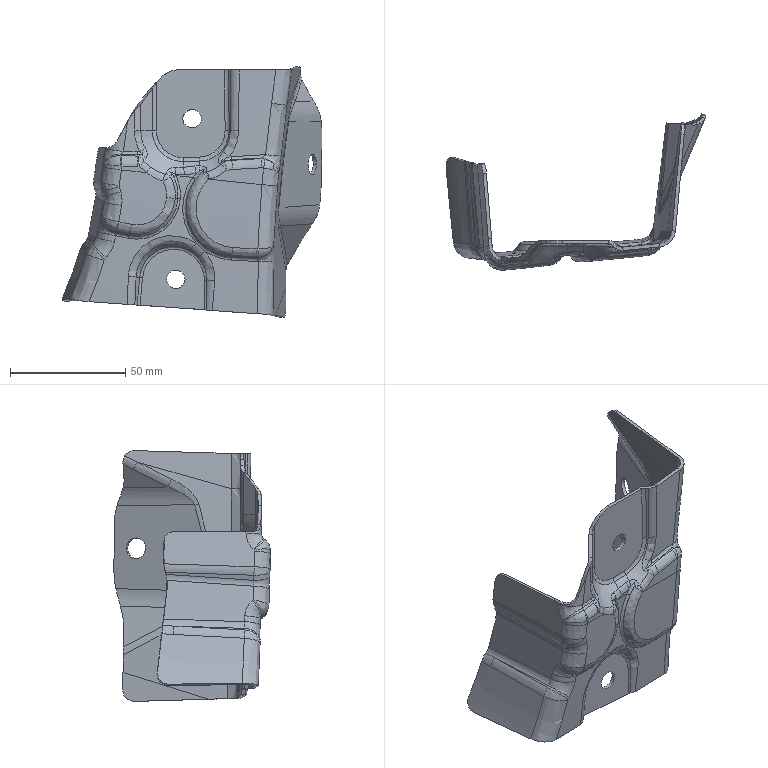Part | STEP file | FNA5401651 | 1 solid | 362 faces | box 112.986 x 67.931 x 109.011 mm | volume 25082 mm3 | spline 298 | cylinder 36 | plane 15 | other 9 | sphere 4 | commonest cylinder face diameters 9 x3 12 x3 14 x3 17092 x3 17095 x3 3 x2